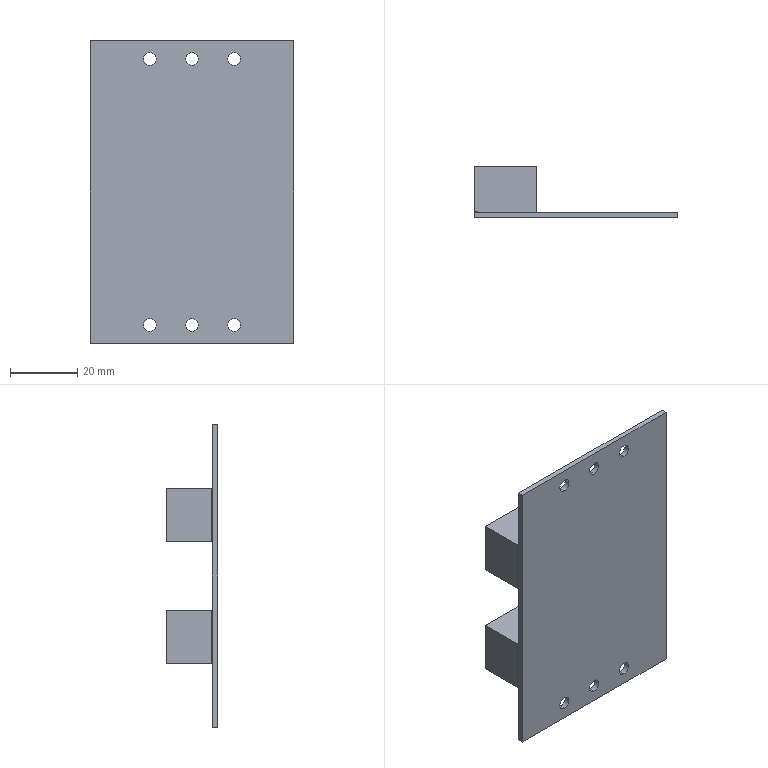Part | SolidWorks | features ICE 3, Extrusion 1 | 1 solid | 32 faces | box 60.4 x 15.3 x 89.7 mm | volume 16562 mm3 | plane 20 | cylinder 12 | commonest cylinder face diameters 3.8 x12
STEP:
#1=CARTESIAN_POINT('',(0.,0.,37.6));
#2=VERTEX_POINT('',#1);
#3=CARTESIAN_POINT('',(0.,0.,41.4));
#4=VERTEX_POINT('',#3);
#5=CARTESIAN_POINT('',(0.,0.,39.5));
#6=DIRECTION('',(0.,1.,0.));
#7=DIRECTION('',(0.,0.,1.));
#8=AXIS2_PLACEMENT_3D('',#5,#6,#7);
#9=CIRCLE('',#8,1.9);
#10=EDGE_CURVE('',#2,#4,#9,.T.);
#11=ORIENTED_EDGE('',*,*,#10,.F.);
#12=CARTESIAN_POINT('',(0.,1.6,37.6));
#13=VERTEX_POINT('',#12);
#14=CARTESIAN_POINT('',(0.,0.,37.6));
#15=DIRECTION('',(0.,1.,0.));
#16=VECTOR('',#15,1000.);
#17=LINE('',#14,#16);
#18=EDGE_CURVE('',#2,#13,#17,.T.);
#19=ORIENTED_EDGE('',*,*,#18,.T.);
#20=CARTESIAN_POINT('',(0.,1.6,41.4));
#21=VERTEX_POINT('',#20);
#22=CARTESIAN_POINT('',(0.,1.6,39.5));
#23=DIRECTION('',(0.,1.,0.));
#24=DIRECTION('',(0.,0.,1.));
#25=AXIS2_PLACEMENT_3D('',#22,#23,#24);
#26=CIRCLE('',#25,1.9);
#27=EDGE_CURVE('',#13,#21,#26,.T.);
#28=ORIENTED_EDGE('',*,*,#27,.T.);
#29=CARTESIAN_POINT('',(0.,0.,41.4));
#30=DIRECTION('',(0.,1.,0.));
#31=VECTOR('',#30,1000.);
#32=LINE('',#29,#31);
#33=EDGE_CURVE('',#4,#21,#32,.T.);
#34=ORIENTED_EDGE('',*,*,#33,.F.);
#35=EDGE_LOOP('',(#11,#19,#28,#34));
#36=FACE_OUTER_BOUND('',#35,.T.);
#37=CARTESIAN_POINT('',(0.,0.,39.5));
#38=DIRECTION('',(0.,1.,0.));
#39=DIRECTION('',(0.,0.,1.));
#40=AXIS2_PLACEMENT_3D('',#37,#38,#39);
#41=CYLINDRICAL_SURFACE('',#40,1.9);
#42=ADVANCED_FACE('',(#36),#41,.F.);
#43=CARTESIAN_POINT('',(0.,0.,-41.4));
#44=VERTEX_POINT('',#43);
#45=CARTESIAN_POINT('',(0.,0.,-37.6));
#46=VERTEX_POINT('',#45);
#47=CARTESIAN_POINT('',(0.,0.,-39.5));
#48=DIRECTION('',(0.,1.,0.));
#49=DIRECTION('',(0.,0.,1.));
#50=AXIS2_PLACEMENT_3D('',#47,#48,#49);
#51=CIRCLE('',#50,1.9);
#52=EDGE_CURVE('',#44,#46,#51,.T.);
#53=ORIENTED_EDGE('',*,*,#52,.F.);
#54=CARTESIAN_POINT('',(0.,1.6,-41.4));
#55=VERTEX_POINT('',#54);
#56=CARTESIAN_POINT('',(0.,0.,-41.4));
#57=DIRECTION('',(0.,1.,0.));
#58=VECTOR('',#57,1000.);
#59=LINE('',#56,#58);
#60=EDGE_CURVE('',#44,#55,#59,.T.);
#61=ORIENTED_EDGE('',*,*,#60,.T.);
#62=CARTESIAN_POINT('',(0.,1.6,-37.6));
#63=VERTEX_POINT('',#62);
#64=CARTESIAN_POINT('',(0.,1.6,-39.5));
#65=DIRECTION('',(0.,1.,0.));
#66=DIRECTION('',(0.,0.,1.));
#67=AXIS2_PLACEMENT_3D('',#64,#65,#66);
#68=CIRCLE('',#67,1.9);
#69=EDGE_CURVE('',#55,#63,#68,.T.);
#70=ORIENTED_EDGE('',*,*,#69,.T.);
#71=CARTESIAN_POINT('',(0.,0.,-37.6));
#72=DIRECTION('',(0.,1.,0.));
#73=VECTOR('',#72,1000.);
#74=LINE('',#71,#73);
#75=EDGE_CURVE('',#46,#63,#74,.T.);
#76=ORIENTED_EDGE('',*,*,#75,.F.);
#77=EDGE_LOOP('',(#53,#61,#70,#76));
#78=FACE_OUTER_BOUND('',#77,.T.);
#79=CARTESIAN_POINT('',(0.,0.,-39.5));
#80=DIRECTION('',(0.,1.,0.));
#81=DIRECTION('',(0.,0.,1.));
#82=AXIS2_PLACEMENT_3D('',#79,#80,#81);
#83=CYLINDRICAL_SURFACE('',#82,1.9);
#84=ADVANCED_FACE('',(#78),#83,.F.);
#85=CARTESIAN_POINT('',(12.5,0.,-41.4));
#86=VERTEX_POINT('',#85);
#87=CARTESIAN_POINT('',(12.5,0.,-37.6));
#88=VERTEX_POINT('',#87);
#89=CARTESIAN_POINT('',(12.5,0.,-39.5));
#90=DIRECTION('',(0.,1.,0.));
#91=DIRECTION('',(0.,0.,1.));
#92=AXIS2_PLACEMENT_3D('',#89,#90,#91);
#93=CIRCLE('',#92,1.9);
#94=EDGE_CURVE('',#86,#88,#93,.T.);
#95=ORIENTED_EDGE('',*,*,#94,.F.);
#96=CARTESIAN_POINT('',(12.5,1.6,-41.4));
#97=VERTEX_POINT('',#96);
#98=CARTESIAN_POINT('',(12.5,0.,-41.4));
#99=DIRECTION('',(0.,1.,0.));
#100=VECTOR('',#99,1000.);
#101=LINE('',#98,#100);
#102=EDGE_CURVE('',#86,#97,#101,.T.);
#103=ORIENTED_EDGE('',*,*,#102,.T.);
#104=CARTESIAN_POINT('',(12.5,1.6,-37.6));
#105=VERTEX_POINT('',#104);
#106=CARTESIAN_POINT('',(12.5,1.6,-39.5));
#107=DIRECTION('',(0.,1.,0.));
#108=DIRECTION('',(0.,0.,1.));
#109=AXIS2_PLACEMENT_3D('',#106,#107,#108);
#110=CIRCLE('',#109,1.9);
#111=EDGE_CURVE('',#97,#105,#110,.T.);
#112=ORIENTED_EDGE('',*,*,#111,.T.);
#113=CARTESIAN_POINT('',(12.5,0.,-37.6));
#114=DIRECTION('',(0.,1.,0.));
#115=VECTOR('',#114,1000.);
#116=LINE('',#113,#115);
#117=EDGE_CURVE('',#88,#105,#116,.T.);
#118=ORIENTED_EDGE('',*,*,#117,.F.);
#119=EDGE_LOOP('',(#95,#103,#112,#118));
#120=FACE_OUTER_BOUND('',#119,.T.);
#121=CARTESIAN_POINT('',(12.5,0.,-39.5));
#122=DIRECTION('',(0.,1.,0.));
#123=DIRECTION('',(0.,0.,1.));
#124=AXIS2_PLACEMENT_3D('',#121,#122,#123);
#125=CYLINDRICAL_SURFACE('',#124,1.9);
#126=ADVANCED_FACE('',(#120),#125,.F.);
#127=CARTESIAN_POINT('',(-12.5,0.,-41.4));
#128=VERTEX_POINT('',#127);
#129=CARTESIAN_POINT('',(-12.5,0.,-37.6));
#130=VERTEX_POINT('',#129);
#131=CARTESIAN_POINT('',(-12.5,0.,-39.5));
#132=DIRECTION('',(0.,1.,0.));
#133=DIRECTION('',(0.,0.,1.));
#134=AXIS2_PLACEMENT_3D('',#131,#132,#133);
#135=CIRCLE('',#134,1.9);
#136=EDGE_CURVE('',#128,#130,#135,.T.);
#137=ORIENTED_EDGE('',*,*,#136,.F.);
#138=CARTESIAN_POINT('',(-12.5,1.6,-41.4));
#139=VERTEX_POINT('',#138);
#140=CARTESIAN_POINT('',(-12.5,0.,-41.4));
#141=DIRECTION('',(0.,1.,0.));
#142=VECTOR('',#141,1000.);
#143=LINE('',#140,#142);
#144=EDGE_CURVE('',#128,#139,#143,.T.);
#145=ORIENTED_EDGE('',*,*,#144,.T.);
#146=CARTESIAN_POINT('',(-12.5,1.6,-37.6));
#147=VERTEX_POINT('',#146);
#148=CARTESIAN_POINT('',(-12.5,1.6,-39.5));
#149=DIRECTION('',(0.,1.,0.));
#150=DIRECTION('',(0.,0.,1.));
#151=AXIS2_PLACEMENT_3D('',#148,#149,#150);
#152=CIRCLE('',#151,1.9);
#153=EDGE_CURVE('',#139,#147,#152,.T.);
#154=ORIENTED_EDGE('',*,*,#153,.T.);
#155=CARTESIAN_POINT('',(-12.5,0.,-37.6));
#156=DIRECTION('',(0.,1.,0.));
#157=VECTOR('',#156,1000.);
#158=LINE('',#155,#157);
#159=EDGE_CURVE('',#130,#147,#158,.T.);
#160=ORIENTED_EDGE('',*,*,#159,.F.);
#161=EDGE_LOOP('',(#137,#145,#154,#160));
#162=FACE_OUTER_BOUND('',#161,.T.);
#163=CARTESIAN_POINT('',(-12.5,0.,-39.5));
#164=DIRECTION('',(0.,1.,0.));
#165=DIRECTION('',(0.,0.,1.));
#166=AXIS2_PLACEMENT_3D('',#163,#164,#165);
#167=CYLINDRICAL_SURFACE('',#166,1.9);
#168=ADVANCED_FACE('',(#162),#167,.F.);
#169=CARTESIAN_POINT('',(12.5,0.,37.6));
#170=VERTEX_POINT('',#169);
#171=CARTESIAN_POINT('',(12.5,0.,41.4));
#172=VERTEX_POINT('',#171);
#173=CARTESIAN_POINT('',(12.5,0.,39.5));
#174=DIRECTION('',(0.,1.,0.));
#175=DIRECTION('',(0.,0.,1.));
#176=AXIS2_PLACEMENT_3D('',#173,#174,#175);
#177=CIRCLE('',#176,1.9);
#178=EDGE_CURVE('',#170,#172,#177,.T.);
#179=ORIENTED_EDGE('',*,*,#178,.F.);
#180=CARTESIAN_POINT('',(12.5,1.6,37.6));
#181=VERTEX_POINT('',#180);
#182=CARTESIAN_POINT('',(12.5,0.,37.6));
#183=DIRECTION('',(0.,1.,0.));
#184=VECTOR('',#183,1000.);
#185=LINE('',#182,#184);
#186=EDGE_CURVE('',#170,#181,#185,.T.);
#187=ORIENTED_EDGE('',*,*,#186,.T.);
#188=CARTESIAN_POINT('',(12.5,1.6,41.4));
#189=VERTEX_POINT('',#188);
#190=CARTESIAN_POINT('',(12.5,1.6,39.5));
#191=DIRECTION('',(0.,1.,0.));
#192=DIRECTION('',(0.,0.,1.));
#193=AXIS2_PLACEMENT_3D('',#190,#191,#192);
#194=CIRCLE('',#193,1.9);
#195=EDGE_CURVE('',#181,#189,#194,.T.);
#196=ORIENTED_EDGE('',*,*,#195,.T.);
#197=CARTESIAN_POINT('',(12.5,0.,41.4));
#198=DIRECTION('',(0.,1.,0.));
#199=VECTOR('',#198,1000.);
#200=LINE('',#197,#199);
#201=EDGE_CURVE('',#172,#189,#200,.T.);
#202=ORIENTED_EDGE('',*,*,#201,.F.);
#203=EDGE_LOOP('',(#179,#187,#196,#202));
#204=FACE_OUTER_BOUND('',#203,.T.);
#205=CARTESIAN_POINT('',(12.5,0.,39.5));
#206=DIRECTION('',(0.,1.,0.));
#207=DIRECTION('',(0.,0.,1.));
#208=AXIS2_PLACEMENT_3D('',#205,#206,#207);
#209=CYLINDRICAL_SURFACE('',#208,1.9);
#210=ADVANCED_FACE('',(#204),#209,.F.);
#211=CARTESIAN_POINT('',(-12.5,0.,37.6));
#212=VERTEX_POINT('',#211);
#213=CARTESIAN_POINT('',(-12.5,0.,41.4));
#214=VERTEX_POINT('',#213);
#215=CARTESIAN_POINT('',(-12.5,0.,39.5));
#216=DIRECTION('',(0.,1.,0.));
#217=DIRECTION('',(0.,0.,1.));
#218=AXIS2_PLACEMENT_3D('',#215,#216,#217);
#219=CIRCLE('',#218,1.9);
#220=EDGE_CURVE('',#212,#214,#219,.T.);
#221=ORIENTED_EDGE('',*,*,#220,.F.);
#222=CARTESIAN_POINT('',(-12.5,1.6,37.6));
#223=VERTEX_POINT('',#222);
#224=CARTESIAN_POINT('',(-12.5,0.,37.6));
#225=DIRECTION('',(0.,1.,0.));
#226=VECTOR('',#225,1000.);
#227=LINE('',#224,#226);
#228=EDGE_CURVE('',#212,#223,#227,.T.);
#229=ORIENTED_EDGE('',*,*,#228,.T.);
#230=CARTESIAN_POINT('',(-12.5,1.6,41.4));
#231=VERTEX_POINT('',#230);
#232=CARTESIAN_POINT('',(-12.5,1.6,39.5));
#233=DIRECTION('',(0.,1.,0.));
#234=DIRECTION('',(0.,0.,1.));
#235=AXIS2_PLACEMENT_3D('',#232,#233,#234);
#236=CIRCLE('',#235,1.9);
#237=EDGE_CURVE('',#223,#231,#236,.T.);
#238=ORIENTED_EDGE('',*,*,#237,.T.);
#239=CARTESIAN_POINT('',(-12.5,0.,41.4));
#240=DIRECTION('',(0.,1.,0.));
#241=VECTOR('',#240,1000.);
#242=LINE('',#239,#241);
#243=EDGE_CURVE('',#214,#231,#242,.T.);
#244=ORIENTED_EDGE('',*,*,#243,.F.);
#245=EDGE_LOOP('',(#221,#229,#238,#244));
#246=FACE_OUTER_BOUND('',#245,.T.);
#247=CARTESIAN_POINT('',(-12.5,0.,39.5));
#248=DIRECTION('',(0.,1.,0.));
#249=DIRECTION('',(0.,0.,1.));
#250=AXIS2_PLACEMENT_3D('',#247,#248,#249);
#251=CYLINDRICAL_SURFACE('',#250,1.9);
#252=ADVANCED_FACE('',(#246),#251,.F.);
#253=CARTESIAN_POINT('',(-30.2,15.3,10.1));
#254=VERTEX_POINT('',#253);
#255=CARTESIAN_POINT('',(-30.2,1.8,10.1));
#256=VERTEX_POINT('',#255);
#257=CARTESIAN_POINT('',(-30.2,15.3,10.1));
#258=DIRECTION('',(0.,-1.,0.));
#259=VECTOR('',#258,1000.);
#260=LINE('',#257,#259);
#261=EDGE_CURVE('',#254,#256,#260,.T.);
#262=ORIENTED_EDGE('',*,*,#261,.T.);
#263=CARTESIAN_POINT('',(-30.2,1.8,25.9));
#264=VERTEX_POINT('',#263);
#265=CARTESIAN_POINT('',(-30.2,1.8,-25.9));
#266=DIRECTION('',(0.,0.,-1.));
#267=VECTOR('',#266,1000.);
#268=LINE('',#265,#267);
#269=EDGE_CURVE('',#264,#256,#268,.T.);
#270=ORIENTED_EDGE('',*,*,#269,.F.);
#271=CARTESIAN_POINT('',(-30.2,15.3,25.9));
#272=VERTEX_POINT('',#271);
#273=CARTESIAN_POINT('',(-30.2,15.3,25.9));
#274=DIRECTION('',(0.,1.,0.));
#275=VECTOR('',#274,1000.);
#276=LINE('',#273,#275);
#277=EDGE_CURVE('',#264,#272,#276,.T.);
#278=ORIENTED_EDGE('',*,*,#277,.T.);
#279=CARTESIAN_POINT('',(-30.2,15.3,10.1));
#280=DIRECTION('',(0.,0.,-1.));
#281=VECTOR('',#280,1000.);
#282=LINE('',#279,#281);
#283=EDGE_CURVE('',#272,#254,#282,.T.);
#284=ORIENTED_EDGE('',*,*,#283,.T.);
#285=EDGE_LOOP('',(#262,#270,#278,#284));
#286=FACE_OUTER_BOUND('',#285,.T.);
#287=CARTESIAN_POINT('',(-30.2,1.6,-44.85));
#288=DIRECTION('',(1.,0.,0.));
#289=DIRECTION('',(0.,0.,-1.));
#290=AXIS2_PLACEMENT_3D('',#287,#288,#289);
#291=PLANE('',#290);
#292=ADVANCED_FACE('',(#286),#291,.F.);
#293=CARTESIAN_POINT('',(-30.2,15.3,-25.9));
#294=VERTEX_POINT('',#293);
#295=CARTESIAN_POINT('',(-30.2,1.8,-25.9));
#296=VERTEX_POINT('',#295);
#297=CARTESIAN_POINT('',(-30.2,15.3,-25.9));
#298=DIRECTION('',(0.,-1.,0.));
#299=VECTOR('',#298,1000.);
#300=LINE('',#297,#299);
#301=EDGE_CURVE('',#294,#296,#300,.T.);
#302=ORIENTED_EDGE('',*,*,#301,.T.);
#303=CARTESIAN_POINT('',(-30.2,1.8,-10.1));
#304=VERTEX_POINT('',#303);
#305=CARTESIAN_POINT('',(-30.2,1.8,-25.9));
#306=DIRECTION('',(0.,0.,-1.));
#307=VECTOR('',#306,1000.);
#308=LINE('',#305,#307);
#309=EDGE_CURVE('',#304,#296,#308,.T.);
#310=ORIENTED_EDGE('',*,*,#309,.F.);
#311=CARTESIAN_POINT('',(-30.2,15.3,-10.1));
#312=VERTEX_POINT('',#311);
#313=CARTESIAN_POINT('',(-30.2,15.3,-10.1));
#314=DIRECTION('',(0.,1.,0.));
#315=VECTOR('',#314,1000.);
#316=LINE('',#313,#315);
#317=EDGE_CURVE('',#304,#312,#316,.T.);
#318=ORIENTED_EDGE('',*,*,#317,.T.);
#319=CARTESIAN_POINT('',(-30.2,15.3,-25.9));
#320=DIRECTION('',(0.,0.,-1.));
#321=VECTOR('',#320,1000.);
#322=LINE('',#319,#321);
#323=EDGE_CURVE('',#312,#294,#322,.T.);
#324=ORIENTED_EDGE('',*,*,#323,.T.);
#325=EDGE_LOOP('',(#302,#310,#318,#324));
#326=FACE_OUTER_BOUND('',#325,.T.);
#327=CARTESIAN_POINT('',(-30.2,1.6,-44.85));
#328=DIRECTION('',(1.,0.,0.));
#329=DIRECTION('',(0.,0.,-1.));
#330=AXIS2_PLACEMENT_3D('',#327,#328,#329);
#331=PLANE('',#330);
#332=ADVANCED_FACE('',(#326),#331,.F.);
#333=CARTESIAN_POINT('',(30.2,0.,44.85));
#334=VERTEX_POINT('',#333);
#335=CARTESIAN_POINT('',(30.2,0.,-44.85));
#336=VERTEX_POINT('',#335);
#337=CARTESIAN_POINT('',(30.2,0.,-44.85));
#338=DIRECTION('',(0.,0.,-1.));
#339=VECTOR('',#338,1000.);
#340=LINE('',#337,#339);
#341=EDGE_CURVE('',#334,#336,#340,.T.);
#342=ORIENTED_EDGE('',*,*,#341,.T.);
#343=CARTESIAN_POINT('',(30.2,1.6,-44.85));
#344=VERTEX_POINT('',#343);
#345=CARTESIAN_POINT('',(30.2,1.6,-44.85));
#346=DIRECTION('',(0.,-1.,0.));
#347=VECTOR('',#346,1000.);
#348=LINE('',#345,#347);
#349=EDGE_CURVE('',#344,#336,#348,.T.);
#350=ORIENTED_EDGE('',*,*,#349,.F.);
#351=CARTESIAN_POINT('',(30.2,1.6,44.85));
#352=VERTEX_POINT('',#351);
#353=CARTESIAN_POINT('',(30.2,1.6,-44.85));
#354=DIRECTION('',(0.,0.,-1.));
#355=VECTOR('',#354,1000.);
#356=LINE('',#353,#355);
#357=EDGE_CURVE('',#352,#344,#356,.T.);
#358=ORIENTED_EDGE('',*,*,#357,.F.);
#359=CARTESIAN_POINT('',(30.2,1.6,44.85));
#360=DIRECTION('',(0.,-1.,0.));
#361=VECTOR('',#360,1000.);
#362=LINE('',#359,#361);
#363=EDGE_CURVE('',#352,#334,#362,.T.);
#364=ORIENTED_EDGE('',*,*,#363,.T.);
#365=EDGE_LOOP('',(#342,#350,#358,#364));
#366=FACE_OUTER_BOUND('',#365,.T.);
#367=CARTESIAN_POINT('',(30.2,1.6,-44.85));
#368=DIRECTION('',(-1.,0.,0.));
#369=DIRECTION('',(0.,0.,1.));
#370=AXIS2_PLACEMENT_3D('',#367,#368,#369);
#371=PLANE('',#370);
#372=ADVANCED_FACE('',(#366),#371,.F.);
#373=CARTESIAN_POINT('',(-30.2,0.,-44.85));
#374=VERTEX_POINT('',#373);
#375=CARTESIAN_POINT('',(-30.2,0.,-44.85));
#376=DIRECTION('',(-1.,0.,0.));
#377=VECTOR('',#376,1000.);
#378=LINE('',#375,#377);
#379=EDGE_CURVE('',#336,#374,#378,.T.);
#380=ORIENTED_EDGE('',*,*,#379,.T.);
#381=CARTESIAN_POINT('',(-30.2,1.6,-44.85));
#382=VERTEX_POINT('',#381);
#383=CARTESIAN_POINT('',(-30.2,1.6,-44.85));
#384=DIRECTION('',(0.,-1.,0.));
#385=VECTOR('',#384,1000.);
#386=LINE('',#383,#385);
#387=EDGE_CURVE('',#382,#374,#386,.T.);
#388=ORIENTED_EDGE('',*,*,#387,.F.);
#389=CARTESIAN_POINT('',(-30.2,1.6,-44.85));
#390=DIRECTION('',(-1.,0.,0.));
#391=VECTOR('',#390,1000.);
#392=LINE('',#389,#391);
#393=EDGE_CURVE('',#344,#382,#392,.T.);
#394=ORIENTED_EDGE('',*,*,#393,.F.);
#395=ORIENTED_EDGE('',*,*,#349,.T.);
#396=EDGE_LOOP('',(#380,#388,#394,#395));
#397=FACE_OUTER_BOUND('',#396,.T.);
#398=CARTESIAN_POINT('',(-30.2,1.6,-44.85));
#399=DIRECTION('',(0.,0.,1.));
#400=DIRECTION('',(1.,0.,0.));
#401=AXIS2_PLACEMENT_3D('',#398,#399,#400);
#402=PLANE('',#401);
#403=ADVANCED_FACE('',(#397),#402,.F.);
#404=CARTESIAN_POINT('',(-30.2,1.6,44.85));
#405=VERTEX_POINT('',#404);
#406=CARTESIAN_POINT('',(-30.2,0.,44.85));
#407=VERTEX_POINT('',#406);
#408=CARTESIAN_POINT('',(-30.2,1.6,44.85));
#409=DIRECTION('',(0.,-1.,0.));
#410=VECTOR('',#409,1000.);
#411=LINE('',#408,#410);
#412=EDGE_CURVE('',#405,#407,#411,.T.);
#413=ORIENTED_EDGE('',*,*,#412,.F.);
#414=CARTESIAN_POINT('',(-30.2,1.6,-44.85));
#415=DIRECTION('',(0.,0.,1.));
#416=VECTOR('',#415,1000.);
#417=LINE('',#414,#416);
#418=EDGE_CURVE('',#382,#405,#417,.T.);
#419=ORIENTED_EDGE('',*,*,#418,.F.);
#420=ORIENTED_EDGE('',*,*,#387,.T.);
#421=CARTESIAN_POINT('',(-30.2,0.,-44.85));
#422=DIRECTION('',(0.,0.,1.));
#423=VECTOR('',#422,1000.);
#424=LINE('',#421,#423);
#425=EDGE_CURVE('',#374,#407,#424,.T.);
#426=ORIENTED_EDGE('',*,*,#425,.T.);
#427=EDGE_LOOP('',(#413,#419,#420,#426));
#428=FACE_OUTER_BOUND('',#427,.T.);
#429=CARTESIAN_POINT('',(-30.2,1.6,-44.85));
#430=DIRECTION('',(1.,0.,0.));
#431=DIRECTION('',(0.,0.,-1.));
#432=AXIS2_PLACEMENT_3D('',#429,#430,#431);
#433=PLANE('',#432);
#434=ADVANCED_FACE('',(#428),#433,.F.);
#435=CARTESIAN_POINT('',(-30.2,0.,44.85));
#436=DIRECTION('',(1.,0.,0.));
#437=VECTOR('',#436,1000.);
#438=LINE('',#435,#437);
#439=EDGE_CURVE('',#407,#334,#438,.T.);
#440=ORIENTED_EDGE('',*,*,#439,.T.);
#441=ORIENTED_EDGE('',*,*,#363,.F.);
#442=CARTESIAN_POINT('',(-30.2,1.6,44.85));
#443=DIRECTION('',(1.,0.,0.));
#444=VECTOR('',#443,1000.);
#445=LINE('',#442,#444);
#446=EDGE_CURVE('',#405,#352,#445,.T.);
#447=ORIENTED_EDGE('',*,*,#446,.F.);
#448=ORIENTED_EDGE('',*,*,#412,.T.);
#449=EDGE_LOOP('',(#440,#441,#447,#448));
#450=FACE_OUTER_BOUND('',#449,.T.);
#451=CARTESIAN_POINT('',(-30.2,1.6,44.85));
#452=DIRECTION('',(0.,0.,-1.));
#453=DIRECTION('',(-1.,0.,0.));
#454=AXIS2_PLACEMENT_3D('',#451,#452,#453);
#455=PLANE('',#454);
#456=ADVANCED_FACE('',(#450),#455,.F.);
#457=CARTESIAN_POINT('',(-11.7,1.6,-10.1));
#458=VERTEX_POINT('',#457);
#459=CARTESIAN_POINT('',(-29.2,1.6,-10.1));
#460=VERTEX_POINT('',#459);
#461=CARTESIAN_POINT('',(-11.7,1.6,-10.1));
#462=DIRECTION('',(-1.,0.,0.));
#463=VECTOR('',#462,1000.);
#464=LINE('',#461,#463);
#465=EDGE_CURVE('',#458,#460,#464,.T.);
#466=ORIENTED_EDGE('',*,*,#465,.T.);
#467=CARTESIAN_POINT('',(-29.2,1.6,-25.9));
#468=VERTEX_POINT('',#467);
#469=CARTESIAN_POINT('',(-29.2,1.6,-25.9));
#470=DIRECTION('',(0.,0.,1.));
#471=VECTOR('',#470,1000.);
#472=LINE('',#469,#471);
#473=EDGE_CURVE('',#468,#460,#472,.T.);
#474=ORIENTED_EDGE('',*,*,#473,.F.);
#475=CARTESIAN_POINT('',(-11.7,1.6,-25.9));
#476=VERTEX_POINT('',#475);
#477=CARTESIAN_POINT('',(-11.7,1.6,-25.9));
#478=DIRECTION('',(-1.,0.,0.));
#479=VECTOR('',#478,1000.);
#480=LINE('',#477,#479);
#481=EDGE_CURVE('',#476,#468,#480,.T.);
#482=ORIENTED_EDGE('',*,*,#481,.F.);
#483=CARTESIAN_POINT('',(-11.7,1.6,-25.9));
#484=DIRECTION('',(0.,0.,1.));
#485=VECTOR('',#484,1000.);
#486=LINE('',#483,#485);
#487=EDGE_CURVE('',#476,#458,#486,.T.);
#488=ORIENTED_EDGE('',*,*,#487,.T.);
#489=EDGE_LOOP('',(#466,#474,#482,#488));
#490=FACE_BOUND('',#489,.T.);
#491=ORIENTED_EDGE('',*,*,#418,.T.);
#492=ORIENTED_EDGE('',*,*,#446,.T.);
#493=ORIENTED_EDGE('',*,*,#357,.T.);
#494=ORIENTED_EDGE('',*,*,#393,.T.);
#495=EDGE_LOOP('',(#491,#492,#493,#494));
#496=FACE_OUTER_BOUND('',#495,.T.);
#497=CARTESIAN_POINT('',(-29.2,1.6,10.1));
#498=VERTEX_POINT('',#497);
#499=CARTESIAN_POINT('',(-29.2,1.6,25.9));
#500=VERTEX_POINT('',#499);
#501=CARTESIAN_POINT('',(-29.2,1.6,-25.9));
#502=DIRECTION('',(0.,0.,1.));
#503=VECTOR('',#502,1000.);
#504=LINE('',#501,#503);
#505=EDGE_CURVE('',#498,#500,#504,.T.);
#506=ORIENTED_EDGE('',*,*,#505,.F.);
#507=CARTESIAN_POINT('',(-11.7,1.6,10.1));
#508=VERTEX_POINT('',#507);
#509=CARTESIAN_POINT('',(-11.7,1.6,10.1));
#510=DIRECTION('',(-1.,0.,0.));
#511=VECTOR('',#510,1000.);
#512=LINE('',#509,#511);
#513=EDGE_CURVE('',#508,#498,#512,.T.);
#514=ORIENTED_EDGE('',*,*,#513,.F.);
#515=CARTESIAN_POINT('',(-11.7,1.6,25.9));
#516=VERTEX_POINT('',#515);
#517=CARTESIAN_POINT('',(-11.7,1.6,10.1));
#518=DIRECTION('',(0.,0.,1.));
#519=VECTOR('',#518,1000.);
#520=LINE('',#517,#519);
#521=EDGE_CURVE('',#508,#516,#520,.T.);
#522=ORIENTED_EDGE('',*,*,#521,.T.);
#523=CARTESIAN_POINT('',(-11.7,1.6,25.9));
#524=DIRECTION('',(-1.,0.,0.));
#525=VECTOR('',#524,1000.);
#526=LINE('',#523,#525);
#527=EDGE_CURVE('',#516,#500,#526,.T.);
#528=ORIENTED_EDGE('',*,*,#527,.T.);
#529=EDGE_LOOP('',(#506,#514,#522,#528));
#530=FACE_BOUND('',#529,.T.);
#531=CARTESIAN_POINT('',(0.,1.6,39.5));
#532=DIRECTION('',(0.,1.,0.));
#533=DIRECTION('',(0.,0.,1.));
#534=AXIS2_PLACEMENT_3D('',#531,#532,#533);
#535=CIRCLE('',#534,1.9);
#536=EDGE_CURVE('',#21,#13,#535,.T.);
#537=ORIENTED_EDGE('',*,*,#536,.F.);
#538=ORIENTED_EDGE('',*,*,#27,.F.);
#539=EDGE_LOOP('',(#537,#538));
#540=FACE_BOUND('',#539,.T.);
#541=CARTESIAN_POINT('',(0.,1.6,-39.5));
#542=DIRECTION('',(0.,1.,0.));
#543=DIRECTION('',(0.,0.,1.));
#544=AXIS2_PLACEMENT_3D('',#541,#542,#543);
#545=CIRCLE('',#544,1.9);
#546=EDGE_CURVE('',#63,#55,#545,.T.);
#547=ORIENTED_EDGE('',*,*,#546,.F.);
#548=ORIENTED_EDGE('',*,*,#69,.F.);
#549=EDGE_LOOP('',(#547,#548));
#550=FACE_BOUND('',#549,.T.);
#551=CARTESIAN_POINT('',(12.5,1.6,-39.5));
#552=DIRECTION('',(0.,1.,0.));
#553=DIRECTION('',(0.,0.,1.));
#554=AXIS2_PLACEMENT_3D('',#551,#552,#553);
#555=CIRCLE('',#554,1.9);
#556=EDGE_CURVE('',#105,#97,#555,.T.);
#557=ORIENTED_EDGE('',*,*,#556,.F.);
#558=ORIENTED_EDGE('',*,*,#111,.F.);
#559=EDGE_LOOP('',(#557,#558));
#560=FACE_BOUND('',#559,.T.);
#561=CARTESIAN_POINT('',(-12.5,1.6,-39.5));
#562=DIRECTION('',(0.,1.,0.));
#563=DIRECTION('',(0.,0.,1.));
#564=AXIS2_PLACEMENT_3D('',#561,#562,#563);
#565=CIRCLE('',#564,1.9);
#566=EDGE_CURVE('',#147,#139,#565,.T.);
#567=ORIENTED_EDGE('',*,*,#566,.F.);
#568=ORIENTED_EDGE('',*,*,#153,.F.);
#569=EDGE_LOOP('',(#567,#568));
#570=FACE_BOUND('',#569,.T.);
#571=CARTESIAN_POINT('',(12.5,1.6,39.5));
#572=DIRECTION('',(0.,1.,0.));
#573=DIRECTION('',(0.,0.,1.));
#574=AXIS2_PLACEMENT_3D('',#571,#572,#573);
#575=CIRCLE('',#574,1.9);
#576=EDGE_CURVE('',#189,#181,#575,.T.);
#577=ORIENTED_EDGE('',*,*,#576,.F.);
#578=ORIENTED_EDGE('',*,*,#195,.F.);
#579=EDGE_LOOP('',(#577,#578));
#580=FACE_BOUND('',#579,.T.);
#581=CARTESIAN_POINT('',(-12.5,1.6,39.5));
#582=DIRECTION('',(0.,1.,0.));
#583=DIRECTION('',(0.,0.,1.));
#584=AXIS2_PLACEMENT_3D('',#581,#582,#583);
#585=CIRCLE('',#584,1.9);
#586=EDGE_CURVE('',#231,#223,#585,.T.);
#587=ORIENTED_EDGE('',*,*,#586,.F.);
#588=ORIENTED_EDGE('',*,*,#237,.F.);
#589=EDGE_LOOP('',(#587,#588));
#590=FACE_BOUND('',#589,.T.);
#591=CARTESIAN_POINT('',(0.,1.6,0.));
#592=DIRECTION('',(0.,1.,0.));
#593=DIRECTION('',(0.,0.,1.));
#594=AXIS2_PLACEMENT_3D('',#591,#592,#593);
#595=PLANE('',#594);
#596=ADVANCED_FACE('',(#490,#496,#530,#540,#550,#560,#570,#580,#590),#595,.T.);
#597=CARTESIAN_POINT('',(0.,0.,39.5));
#598=DIRECTION('',(0.,1.,0.));
#599=DIRECTION('',(0.,0.,1.));
#600=AXIS2_PLACEMENT_3D('',#597,#598,#599);
#601=CIRCLE('',#600,1.9);
#602=EDGE_CURVE('',#4,#2,#601,.T.);
#603=ORIENTED_EDGE('',*,*,#602,.T.);
#604=ORIENTED_EDGE('',*,*,#10,.T.);
#605=EDGE_LOOP('',(#603,#604));
#606=FACE_BOUND('',#605,.T.);
#607=CARTESIAN_POINT('',(0.,0.,-39.5));
#608=DIRECTION('',(0.,1.,0.));
#609=DIRECTION('',(0.,0.,1.));
#610=AXIS2_PLACEMENT_3D('',#607,#608,#609);
#611=CIRCLE('',#610,1.9);
#612=EDGE_CURVE('',#46,#44,#611,.T.);
#613=ORIENTED_EDGE('',*,*,#612,.T.);
#614=ORIENTED_EDGE('',*,*,#52,.T.);
#615=EDGE_LOOP('',(#613,#614));
#616=FACE_BOUND('',#615,.T.);
#617=CARTESIAN_POINT('',(12.5,0.,-39.5));
#618=DIRECTION('',(0.,1.,0.));
#619=DIRECTION('',(0.,0.,1.));
#620=AXIS2_PLACEMENT_3D('',#617,#618,#619);
#621=CIRCLE('',#620,1.9);
#622=EDGE_CURVE('',#88,#86,#621,.T.);
#623=ORIENTED_EDGE('',*,*,#622,.T.);
#624=ORIENTED_EDGE('',*,*,#94,.T.);
#625=EDGE_LOOP('',(#623,#624));
#626=FACE_BOUND('',#625,.T.);
#627=CARTESIAN_POINT('',(-12.5,0.,-39.5));
#628=DIRECTION('',(0.,1.,0.));
#629=DIRECTION('',(0.,0.,1.));
#630=AXIS2_PLACEMENT_3D('',#627,#628,#629);
#631=CIRCLE('',#630,1.9);
#632=EDGE_CURVE('',#130,#128,#631,.T.);
#633=ORIENTED_EDGE('',*,*,#632,.T.);
#634=ORIENTED_EDGE('',*,*,#136,.T.);
#635=EDGE_LOOP('',(#633,#634));
#636=FACE_BOUND('',#635,.T.);
#637=CARTESIAN_POINT('',(12.5,0.,39.5));
#638=DIRECTION('',(0.,1.,0.));
#639=DIRECTION('',(0.,0.,1.));
#640=AXIS2_PLACEMENT_3D('',#637,#638,#639);
#641=CIRCLE('',#640,1.9);
#642=EDGE_CURVE('',#172,#170,#641,.T.);
#643=ORIENTED_EDGE('',*,*,#642,.T.);
#644=ORIENTED_EDGE('',*,*,#178,.T.);
#645=EDGE_LOOP('',(#643,#644));
#646=FACE_BOUND('',#645,.T.);
#647=CARTESIAN_POINT('',(-12.5,0.,39.5));
#648=DIRECTION('',(0.,1.,0.));
#649=DIRECTION('',(0.,0.,1.));
#650=AXIS2_PLACEMENT_3D('',#647,#648,#649);
#651=CIRCLE('',#650,1.9);
#652=EDGE_CURVE('',#214,#212,#651,.T.);
#653=ORIENTED_EDGE('',*,*,#652,.T.);
#654=ORIENTED_EDGE('',*,*,#220,.T.);
#655=EDGE_LOOP('',(#653,#654));
#656=FACE_BOUND('',#655,.T.);
#657=ORIENTED_EDGE('',*,*,#341,.F.);
#658=ORIENTED_EDGE('',*,*,#439,.F.);
#659=ORIENTED_EDGE('',*,*,#425,.F.);
#660=ORIENTED_EDGE('',*,*,#379,.F.);
#661=EDGE_LOOP('',(#657,#658,#659,#660));
#662=FACE_OUTER_BOUND('',#661,.T.);
#663=CARTESIAN_POINT('',(0.,0.,0.));
#664=DIRECTION('',(0.,1.,0.));
#665=DIRECTION('',(0.,0.,1.));
#666=AXIS2_PLACEMENT_3D('',#663,#664,#665);
#667=PLANE('',#666);
#668=ADVANCED_FACE('',(#606,#616,#626,#636,#646,#656,#662),#667,.F.);
#669=ORIENTED_EDGE('',*,*,#228,.F.);
#670=ORIENTED_EDGE('',*,*,#652,.F.);
#671=ORIENTED_EDGE('',*,*,#243,.T.);
#672=ORIENTED_EDGE('',*,*,#586,.T.);
#673=EDGE_LOOP('',(#669,#670,#671,#672));
#674=FACE_OUTER_BOUND('',#673,.T.);
#675=CARTESIAN_POINT('',(-12.5,0.,39.5));
#676=DIRECTION('',(0.,1.,0.));
#677=DIRECTION('',(0.,0.,1.));
#678=AXIS2_PLACEMENT_3D('',#675,#676,#677);
#679=CYLINDRICAL_SURFACE('',#678,1.9);
#680=ADVANCED_FACE('',(#674),#679,.F.);
#681=ORIENTED_EDGE('',*,*,#186,.F.);
#682=ORIENTED_EDGE('',*,*,#642,.F.);
#683=ORIENTED_EDGE('',*,*,#201,.T.);
#684=ORIENTED_EDGE('',*,*,#576,.T.);
#685=EDGE_LOOP('',(#681,#682,#683,#684));
#686=FACE_OUTER_BOUND('',#685,.T.);
#687=CARTESIAN_POINT('',(12.5,0.,39.5));
#688=DIRECTION('',(0.,1.,0.));
#689=DIRECTION('',(0.,0.,1.));
#690=AXIS2_PLACEMENT_3D('',#687,#688,#689);
#691=CYLINDRICAL_SURFACE('',#690,1.9);
#692=ADVANCED_FACE('',(#686),#691,.F.);
#693=ORIENTED_EDGE('',*,*,#144,.F.);
#694=ORIENTED_EDGE('',*,*,#632,.F.);
#695=ORIENTED_EDGE('',*,*,#159,.T.);
#696=ORIENTED_EDGE('',*,*,#566,.T.);
#697=EDGE_LOOP('',(#693,#694,#695,#696));
#698=FACE_OUTER_BOUND('',#697,.T.);
#699=CARTESIAN_POINT('',(-12.5,0.,-39.5));
#700=DIRECTION('',(0.,1.,0.));
#701=DIRECTION('',(0.,0.,1.));
#702=AXIS2_PLACEMENT_3D('',#699,#700,#701);
#703=CYLINDRICAL_SURFACE('',#702,1.9);
#704=ADVANCED_FACE('',(#698),#703,.F.);
#705=ORIENTED_EDGE('',*,*,#102,.F.);
#706=ORIENTED_EDGE('',*,*,#622,.F.);
#707=ORIENTED_EDGE('',*,*,#117,.T.);
#708=ORIENTED_EDGE('',*,*,#556,.T.);
#709=EDGE_LOOP('',(#705,#706,#707,#708));
#710=FACE_OUTER_BOUND('',#709,.T.);
#711=CARTESIAN_POINT('',(12.5,0.,-39.5));
#712=DIRECTION('',(0.,1.,0.));
#713=DIRECTION('',(0.,0.,1.));
#714=AXIS2_PLACEMENT_3D('',#711,#712,#713);
#715=CYLINDRICAL_SURFACE('',#714,1.9);
#716=ADVANCED_FACE('',(#710),#715,.F.);
#717=ORIENTED_EDGE('',*,*,#60,.F.);
#718=ORIENTED_EDGE('',*,*,#612,.F.);
#719=ORIENTED_EDGE('',*,*,#75,.T.);
#720=ORIENTED_EDGE('',*,*,#546,.T.);
#721=EDGE_LOOP('',(#717,#718,#719,#720));
#722=FACE_OUTER_BOUND('',#721,.T.);
#723=CARTESIAN_POINT('',(0.,0.,-39.5));
#724=DIRECTION('',(0.,1.,0.));
#725=DIRECTION('',(0.,0.,1.));
#726=AXIS2_PLACEMENT_3D('',#723,#724,#725);
#727=CYLINDRICAL_SURFACE('',#726,1.9);
#728=ADVANCED_FACE('',(#722),#727,.F.);
#729=ORIENTED_EDGE('',*,*,#18,.F.);
#730=ORIENTED_EDGE('',*,*,#602,.F.);
#731=ORIENTED_EDGE('',*,*,#33,.T.);
#732=ORIENTED_EDGE('',*,*,#536,.T.);
#733=EDGE_LOOP('',(#729,#730,#731,#732));
#734=FACE_OUTER_BOUND('',#733,.T.);
#735=CARTESIAN_POINT('',(0.,0.,39.5));
#736=DIRECTION('',(0.,1.,0.));
#737=DIRECTION('',(0.,0.,1.));
#738=AXIS2_PLACEMENT_3D('',#735,#736,#737);
#739=CYLINDRICAL_SURFACE('',#738,1.9);
#740=ADVANCED_FACE('',(#734),#739,.F.);
#741=CARTESIAN_POINT('',(-29.2,1.8,10.1));
#742=VERTEX_POINT('',#741);
#743=CARTESIAN_POINT('',(-11.7,1.8,10.1));
#744=DIRECTION('',(1.,0.,0.));
#745=VECTOR('',#744,1000.);
#746=LINE('',#743,#745);
#747=EDGE_CURVE('',#256,#742,#746,.T.);
#748=ORIENTED_EDGE('',*,*,#747,.F.);
#749=ORIENTED_EDGE('',*,*,#261,.F.);
#750=CARTESIAN_POINT('',(-11.7,15.3,10.1));
#751=VERTEX_POINT('',#750);
#752=CARTESIAN_POINT('',(-11.7,15.3,10.1));
#753=DIRECTION('',(-1.,0.,0.));
#754=VECTOR('',#753,1000.);
#755=LINE('',#752,#754);
#756=EDGE_CURVE('',#751,#254,#755,.T.);
#757=ORIENTED_EDGE('',*,*,#756,.F.);
#758=CARTESIAN_POINT('',(-11.7,15.3,10.1));
#759=DIRECTION('',(0.,-1.,0.));
#760=VECTOR('',#759,1000.);
#761=LINE('',#758,#760);
#762=EDGE_CURVE('',#751,#508,#761,.T.);
#763=ORIENTED_EDGE('',*,*,#762,.T.);
#764=ORIENTED_EDGE('',*,*,#513,.T.);
#765=CARTESIAN_POINT('',(-29.2,15.3,10.1));
#766=DIRECTION('',(0.,-1.,0.));
#767=VECTOR('',#766,1000.);
#768=LINE('',#765,#767);
#769=EDGE_CURVE('',#742,#498,#768,.T.);
#770=ORIENTED_EDGE('',*,*,#769,.F.);
#771=EDGE_LOOP('',(#748,#749,#757,#763,#764,#770));
#772=FACE_OUTER_BOUND('',#771,.T.);
#773=CARTESIAN_POINT('',(-11.7,15.3,10.1));
#774=DIRECTION('',(0.,0.,-1.));
#775=DIRECTION('',(0.,1.,0.));
#776=AXIS2_PLACEMENT_3D('',#773,#774,#775);
#777=PLANE('',#776);
#778=ADVANCED_FACE('',(#772),#777,.T.);
#779=ORIENTED_EDGE('',*,*,#283,.F.);
#780=CARTESIAN_POINT('',(-11.7,15.3,25.9));
#781=VERTEX_POINT('',#780);
#782=CARTESIAN_POINT('',(-11.7,15.3,25.9));
#783=DIRECTION('',(-1.,0.,0.));
#784=VECTOR('',#783,1000.);
#785=LINE('',#782,#784);
#786=EDGE_CURVE('',#781,#272,#785,.T.);
#787=ORIENTED_EDGE('',*,*,#786,.F.);
#788=CARTESIAN_POINT('',(-11.7,15.3,10.1));
#789=DIRECTION('',(0.,0.,-1.));
#790=VECTOR('',#789,1000.);
#791=LINE('',#788,#790);
#792=EDGE_CURVE('',#781,#751,#791,.T.);
#793=ORIENTED_EDGE('',*,*,#792,.T.);
#794=ORIENTED_EDGE('',*,*,#756,.T.);
#795=EDGE_LOOP('',(#779,#787,#793,#794));
#796=FACE_OUTER_BOUND('',#795,.T.);
#797=CARTESIAN_POINT('',(-11.7,15.3,10.1));
#798=DIRECTION('',(0.,1.,0.));
#799=DIRECTION('',(0.,0.,1.));
#800=AXIS2_PLACEMENT_3D('',#797,#798,#799);
#801=PLANE('',#800);
#802=ADVANCED_FACE('',(#796),#801,.T.);
#803=CARTESIAN_POINT('',(-29.2,1.8,25.9));
#804=VERTEX_POINT('',#803);
#805=CARTESIAN_POINT('',(-29.2,1.8,25.9));
#806=DIRECTION('',(-1.,0.,0.));
#807=VECTOR('',#806,1000.);
#808=LINE('',#805,#807);
#809=EDGE_CURVE('',#804,#264,#808,.T.);
#810=ORIENTED_EDGE('',*,*,#809,.F.);
#811=CARTESIAN_POINT('',(-29.2,1.6,25.9));
#812=DIRECTION('',(0.,1.,0.));
#813=VECTOR('',#812,1000.);
#814=LINE('',#811,#813);
#815=EDGE_CURVE('',#500,#804,#814,.T.);
#816=ORIENTED_EDGE('',*,*,#815,.F.);
#817=ORIENTED_EDGE('',*,*,#527,.F.);
#818=CARTESIAN_POINT('',(-11.7,15.3,25.9));
#819=DIRECTION('',(0.,1.,0.));
#820=VECTOR('',#819,1000.);
#821=LINE('',#818,#820);
#822=EDGE_CURVE('',#516,#781,#821,.T.);
#823=ORIENTED_EDGE('',*,*,#822,.T.);
#824=ORIENTED_EDGE('',*,*,#786,.T.);
#825=ORIENTED_EDGE('',*,*,#277,.F.);
#826=EDGE_LOOP('',(#810,#816,#817,#823,#824,#825));
#827=FACE_OUTER_BOUND('',#826,.T.);
#828=CARTESIAN_POINT('',(-11.7,15.3,25.9));
#829=DIRECTION('',(0.,0.,1.));
#830=DIRECTION('',(0.,-1.,0.));
#831=AXIS2_PLACEMENT_3D('',#828,#829,#830);
#832=PLANE('',#831);
#833=ADVANCED_FACE('',(#827),#832,.T.);
#834=ORIENTED_EDGE('',*,*,#762,.F.);
#835=ORIENTED_EDGE('',*,*,#792,.F.);
#836=ORIENTED_EDGE('',*,*,#822,.F.);
#837=ORIENTED_EDGE('',*,*,#521,.F.);
#838=EDGE_LOOP('',(#834,#835,#836,#837));
#839=FACE_OUTER_BOUND('',#838,.T.);
#840=CARTESIAN_POINT('',(-11.7,0.,0.));
#841=DIRECTION('',(-1.,0.,0.));
#842=DIRECTION('',(0.,0.,1.));
#843=AXIS2_PLACEMENT_3D('',#840,#841,#842);
#844=PLANE('',#843);
#845=ADVANCED_FACE('',(#839),#844,.F.);
#846=CARTESIAN_POINT('',(-29.2,1.8,-25.9));
#847=VERTEX_POINT('',#846);
#848=CARTESIAN_POINT('',(-29.2,1.8,-25.9));
#849=DIRECTION('',(-1.,0.,0.));
#850=VECTOR('',#849,1000.);
#851=LINE('',#848,#850);
#852=EDGE_CURVE('',#847,#296,#851,.T.);
#853=ORIENTED_EDGE('',*,*,#852,.T.);
#854=ORIENTED_EDGE('',*,*,#301,.F.);
#855=CARTESIAN_POINT('',(-11.7,15.3,-25.9));
#856=VERTEX_POINT('',#855);
#857=CARTESIAN_POINT('',(-11.7,15.3,-25.9));
#858=DIRECTION('',(-1.,0.,0.));
#859=VECTOR('',#858,1000.);
#860=LINE('',#857,#859);
#861=EDGE_CURVE('',#856,#294,#860,.T.);
#862=ORIENTED_EDGE('',*,*,#861,.F.);
#863=CARTESIAN_POINT('',(-11.7,15.3,-25.9));
#864=DIRECTION('',(0.,-1.,0.));
#865=VECTOR('',#864,1000.);
#866=LINE('',#863,#865);
#867=EDGE_CURVE('',#856,#476,#866,.T.);
#868=ORIENTED_EDGE('',*,*,#867,.T.);
#869=ORIENTED_EDGE('',*,*,#481,.T.);
#870=CARTESIAN_POINT('',(-29.2,1.6,-25.9));
#871=DIRECTION('',(0.,-1.,0.));
#872=VECTOR('',#871,1000.);
#873=LINE('',#870,#872);
#874=EDGE_CURVE('',#847,#468,#873,.T.);
#875=ORIENTED_EDGE('',*,*,#874,.F.);
#876=EDGE_LOOP('',(#853,#854,#862,#868,#869,#875));
#877=FACE_OUTER_BOUND('',#876,.T.);
#878=CARTESIAN_POINT('',(-11.7,15.3,-25.9));
#879=DIRECTION('',(0.,0.,-1.));
#880=DIRECTION('',(0.,1.,0.));
#881=AXIS2_PLACEMENT_3D('',#878,#879,#880);
#882=PLANE('',#881);
#883=ADVANCED_FACE('',(#877),#882,.T.);
#884=ORIENTED_EDGE('',*,*,#323,.F.);
#885=CARTESIAN_POINT('',(-11.7,15.3,-10.1));
#886=VERTEX_POINT('',#885);
#887=CARTESIAN_POINT('',(-11.7,15.3,-10.1));
#888=DIRECTION('',(-1.,0.,0.));
#889=VECTOR('',#888,1000.);
#890=LINE('',#887,#889);
#891=EDGE_CURVE('',#886,#312,#890,.T.);
#892=ORIENTED_EDGE('',*,*,#891,.F.);
#893=CARTESIAN_POINT('',(-11.7,15.3,-25.9));
#894=DIRECTION('',(0.,0.,-1.));
#895=VECTOR('',#894,1000.);
#896=LINE('',#893,#895);
#897=EDGE_CURVE('',#886,#856,#896,.T.);
#898=ORIENTED_EDGE('',*,*,#897,.T.);
#899=ORIENTED_EDGE('',*,*,#861,.T.);
#900=EDGE_LOOP('',(#884,#892,#898,#899));
#901=FACE_OUTER_BOUND('',#900,.T.);
#902=CARTESIAN_POINT('',(-11.7,15.3,-25.9));
#903=DIRECTION('',(0.,1.,0.));
#904=DIRECTION('',(0.,0.,1.));
#905=AXIS2_PLACEMENT_3D('',#902,#903,#904);
#906=PLANE('',#905);
#907=ADVANCED_FACE('',(#901),#906,.T.);
#908=CARTESIAN_POINT('',(-29.2,1.8,-10.1));
#909=VERTEX_POINT('',#908);
#910=CARTESIAN_POINT('',(-11.7,1.8,-10.1));
#911=DIRECTION('',(-1.,0.,0.));
#912=VECTOR('',#911,1000.);
#913=LINE('',#910,#912);
#914=EDGE_CURVE('',#909,#304,#913,.T.);
#915=ORIENTED_EDGE('',*,*,#914,.F.);
#916=CARTESIAN_POINT('',(-29.2,15.3,-10.1));
#917=DIRECTION('',(0.,1.,0.));
#918=VECTOR('',#917,1000.);
#919=LINE('',#916,#918);
#920=EDGE_CURVE('',#460,#909,#919,.T.);
#921=ORIENTED_EDGE('',*,*,#920,.F.);
#922=ORIENTED_EDGE('',*,*,#465,.F.);
#923=CARTESIAN_POINT('',(-11.7,15.3,-10.1));
#924=DIRECTION('',(0.,1.,0.));
#925=VECTOR('',#924,1000.);
#926=LINE('',#923,#925);
#927=EDGE_CURVE('',#458,#886,#926,.T.);
#928=ORIENTED_EDGE('',*,*,#927,.T.);
#929=ORIENTED_EDGE('',*,*,#891,.T.);
#930=ORIENTED_EDGE('',*,*,#317,.F.);
#931=EDGE_LOOP('',(#915,#921,#922,#928,#929,#930));
#932=FACE_OUTER_BOUND('',#931,.T.);
#933=CARTESIAN_POINT('',(-11.7,15.3,-10.1));
#934=DIRECTION('',(0.,0.,1.));
#935=DIRECTION('',(0.,-1.,0.));
#936=AXIS2_PLACEMENT_3D('',#933,#934,#935);
#937=PLANE('',#936);
#938=ADVANCED_FACE('',(#932),#937,.T.);
#939=ORIENTED_EDGE('',*,*,#867,.F.);
#940=ORIENTED_EDGE('',*,*,#897,.F.);
#941=ORIENTED_EDGE('',*,*,#927,.F.);
#942=ORIENTED_EDGE('',*,*,#487,.F.);
#943=EDGE_LOOP('',(#939,#940,#941,#942));
#944=FACE_OUTER_BOUND('',#943,.T.);
#945=CARTESIAN_POINT('',(-11.7,0.,0.));
#946=DIRECTION('',(-1.,0.,0.));
#947=DIRECTION('',(0.,0.,1.));
#948=AXIS2_PLACEMENT_3D('',#945,#946,#947);
#949=PLANE('',#948);
#950=ADVANCED_FACE('',(#944),#949,.F.);
#951=ORIENTED_EDGE('',*,*,#920,.T.);
#952=CARTESIAN_POINT('',(-29.2,1.8,-25.9));
#953=DIRECTION('',(0.,0.,-1.));
#954=VECTOR('',#953,1000.);
#955=LINE('',#952,#954);
#956=EDGE_CURVE('',#909,#847,#955,.T.);
#957=ORIENTED_EDGE('',*,*,#956,.T.);
#958=ORIENTED_EDGE('',*,*,#874,.T.);
#959=ORIENTED_EDGE('',*,*,#473,.T.);
#960=EDGE_LOOP('',(#951,#957,#958,#959));
#961=FACE_OUTER_BOUND('',#960,.T.);
#962=CARTESIAN_POINT('',(-29.2,0.,0.));
#963=DIRECTION('',(1.,0.,0.));
#964=DIRECTION('',(0.,0.,-1.));
#965=AXIS2_PLACEMENT_3D('',#962,#963,#964);
#966=PLANE('',#965);
#967=ADVANCED_FACE('',(#961),#966,.F.);
#968=ORIENTED_EDGE('',*,*,#914,.T.);
#969=ORIENTED_EDGE('',*,*,#309,.T.);
#970=ORIENTED_EDGE('',*,*,#852,.F.);
#971=ORIENTED_EDGE('',*,*,#956,.F.);
#972=EDGE_LOOP('',(#968,#969,#970,#971));
#973=FACE_OUTER_BOUND('',#972,.T.);
#974=CARTESIAN_POINT('',(-29.2,1.8,-25.9));
#975=DIRECTION('',(0.,1.,0.));
#976=DIRECTION('',(0.,0.,1.));
#977=AXIS2_PLACEMENT_3D('',#974,#975,#976);
#978=PLANE('',#977);
#979=ADVANCED_FACE('',(#973),#978,.F.);
#980=ORIENTED_EDGE('',*,*,#747,.T.);
#981=CARTESIAN_POINT('',(-29.2,1.8,-25.9));
#982=DIRECTION('',(0.,0.,-1.));
#983=VECTOR('',#982,1000.);
#984=LINE('',#981,#983);
#985=EDGE_CURVE('',#804,#742,#984,.T.);
#986=ORIENTED_EDGE('',*,*,#985,.F.);
#987=ORIENTED_EDGE('',*,*,#809,.T.);
#988=ORIENTED_EDGE('',*,*,#269,.T.);
#989=EDGE_LOOP('',(#980,#986,#987,#988));
#990=FACE_OUTER_BOUND('',#989,.T.);
#991=CARTESIAN_POINT('',(-29.2,1.8,-25.9));
#992=DIRECTION('',(0.,1.,0.));
#993=DIRECTION('',(0.,0.,1.));
#994=AXIS2_PLACEMENT_3D('',#991,#992,#993);
#995=PLANE('',#994);
#996=ADVANCED_FACE('',(#990),#995,.F.);
#997=ORIENTED_EDGE('',*,*,#769,.T.);
#998=ORIENTED_EDGE('',*,*,#505,.T.);
#999=ORIENTED_EDGE('',*,*,#815,.T.);
#1000=ORIENTED_EDGE('',*,*,#985,.T.);
#1001=EDGE_LOOP('',(#997,#998,#999,#1000));
#1002=FACE_OUTER_BOUND('',#1001,.T.);
#1003=CARTESIAN_POINT('',(-29.2,0.,0.));
#1004=DIRECTION('',(1.,0.,0.));
#1005=DIRECTION('',(0.,0.,-1.));
#1006=AXIS2_PLACEMENT_3D('',#1003,#1004,#1005);
#1007=PLANE('',#1006);
#1008=ADVANCED_FACE('',(#1002),#1007,.F.);
#1009=CLOSED_SHELL('',(#42,#84,#126,#168,#210,#252,#292,#332,#372,#403,#434,#456,#596,#668,#680,#692,#704,#716,#728,#740,#778,#802,#833,#845,#883,#907,#938,#950,#967,#979,#996,#1008));
#1010=MANIFOLD_SOLID_BREP('',#1009);
#1011=CARTESIAN_POINT('',(0.,0.,0.));
#1012=DIRECTION('',(0.,0.,1.));
#1013=DIRECTION('',(1.,0.,0.));
#1014=AXIS2_PLACEMENT_3D('',#1011,#1012,#1013);
#1015=(LENGTH_UNIT()NAMED_UNIT(*)SI_UNIT(.MILLI.,.METRE.));
#1016=UNCERTAINTY_MEASURE_WITH_UNIT(LENGTH_MEASURE(0.00001),#1015,'','');
#1017=(NAMED_UNIT(*)PLANE_ANGLE_UNIT()SI_UNIT($,.RADIAN.));
#1018=(NAMED_UNIT(*)SI_UNIT($,.STERADIAN.)SOLID_ANGLE_UNIT());
#1019=(GEOMETRIC_REPRESENTATION_CONTEXT(3)GLOBAL_UNCERTAINTY_ASSIGNED_CONTEXT((#1016))GLOBAL_UNIT_ASSIGNED_CONTEXT((#1015,#1017,#1018))REPRESENTATION_CONTEXT('',''));
#1020=ADVANCED_BREP_SHAPE_REPRESENTATION('',(#1010,#1014),#1019);